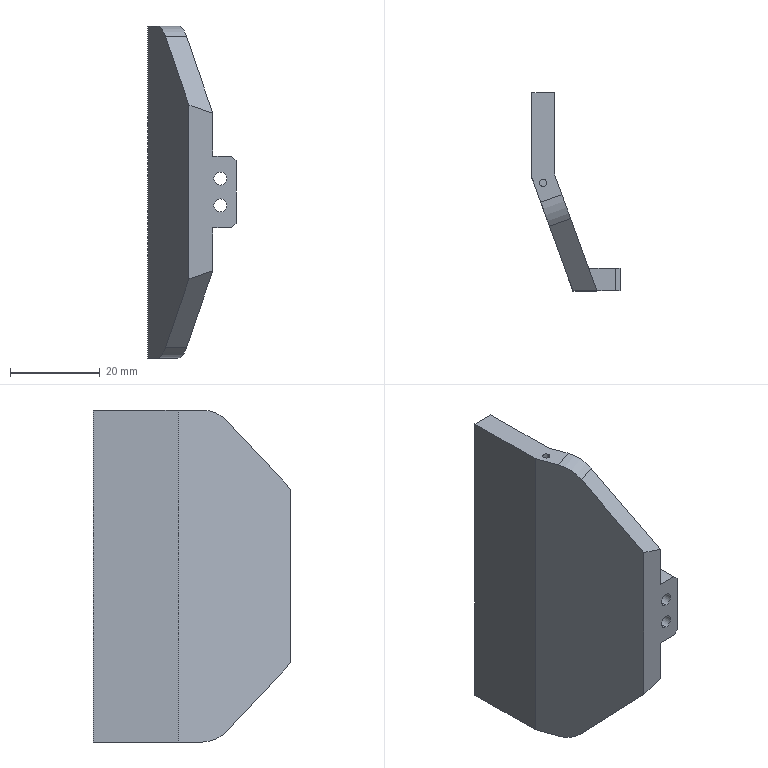NC program | NX | posted with a generic post | part box 19.643 x 44.061 x 74 mm
Whole program:
N10 G17 G21 G94 G90
(DRILLING_1 , TOOL : D4点钻)
N12 T05 M6
N14 G54
N16 G17 G0 G90 X3. Y-3.5 B0. C0. S3000 M3
N18 G43 Z20. H5
N20 G94 G81 G98 Z-1.45 F200. R2.
N22 X-3.
N24 G80
N26 G0 X-3. Y-3.5 Z20.
N28 M5
(DRILLING_1_COPY , TOOL : D2.9钻头)
N30 T08 M6
N32 G54
N34 G17 G0 G90 X3. Y-3.5 B0. C0. S3000 M3
N36 G43 Z20. H8
N38 G94 G81 G98 Z-7. F200. R2.
N40 X-3.
N42 G80
N44 G0 X-3. Y-3.5 Z20.
N46 M5
N48 M2